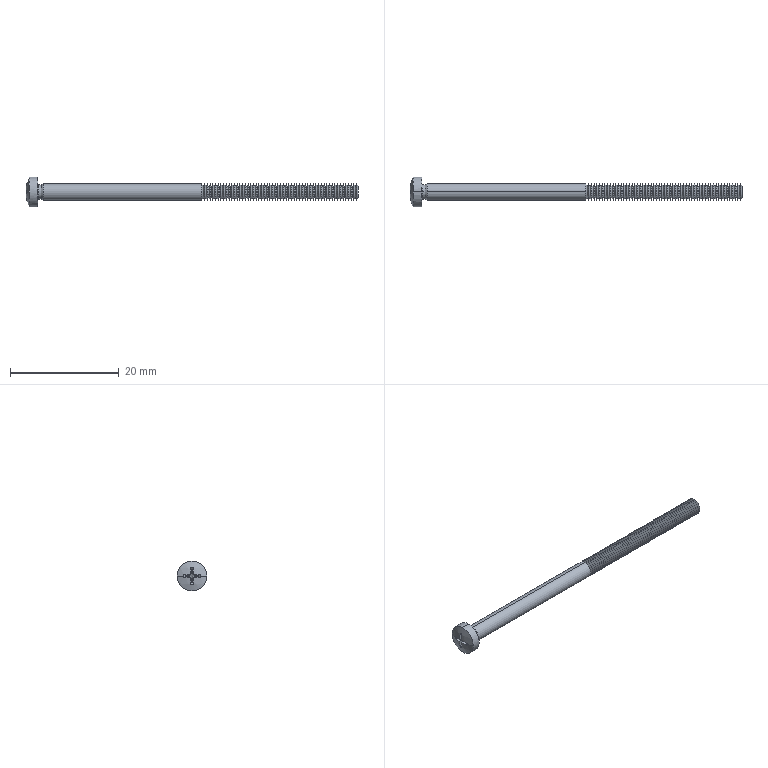Part | SolidWorks | features BaseBody 1 | 1 solid | 256 faces | box 61.141 x 5.5 x 5.5 mm | volume 405.719 mm3 | cone 232 | plane 14 | cylinder 6 | torus 2 | sphere 2 | commonest cylinder face diameters 2.598 x2 3 x2 5.5 x2